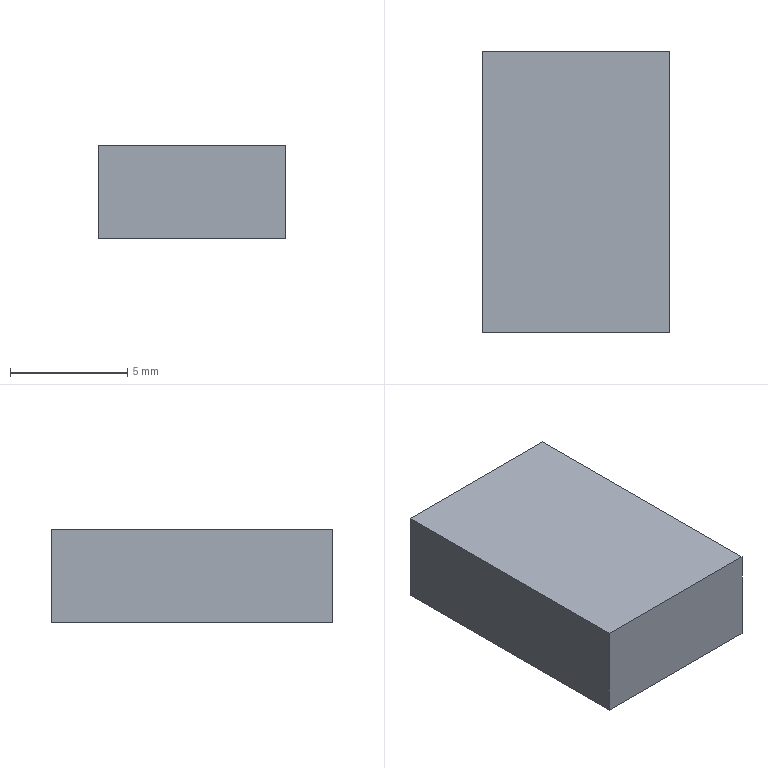Part | SolidWorks | features BaseBody 1 | 1 solid | 6 faces | box 8 x 12 x 4 mm | volume 384 mm3 | plane 6
STEP:
#1=CARTESIAN_POINT('',(4.,-6.,-2.));
#2=VERTEX_POINT('',#1);
#3=CARTESIAN_POINT('',(4.,6.,-2.));
#4=VERTEX_POINT('',#3);
#5=CARTESIAN_POINT('',(4.,-6.,-2.));
#6=DIRECTION('',(0.,1.,0.));
#7=VECTOR('',#6,1000.);
#8=LINE('',#5,#7);
#9=EDGE_CURVE('',#2,#4,#8,.T.);
#10=ORIENTED_EDGE('',*,*,#9,.F.);
#11=CARTESIAN_POINT('',(-4.,-6.,-2.));
#12=VERTEX_POINT('',#11);
#13=CARTESIAN_POINT('',(-4.,-6.,-2.));
#14=DIRECTION('',(1.,0.,0.));
#15=VECTOR('',#14,1000.);
#16=LINE('',#13,#15);
#17=EDGE_CURVE('',#12,#2,#16,.T.);
#18=ORIENTED_EDGE('',*,*,#17,.F.);
#19=CARTESIAN_POINT('',(-4.,6.,-2.));
#20=VERTEX_POINT('',#19);
#21=CARTESIAN_POINT('',(-4.,-6.,-2.));
#22=DIRECTION('',(0.,-1.,0.));
#23=VECTOR('',#22,1000.);
#24=LINE('',#21,#23);
#25=EDGE_CURVE('',#20,#12,#24,.T.);
#26=ORIENTED_EDGE('',*,*,#25,.F.);
#27=CARTESIAN_POINT('',(-4.,6.,-2.));
#28=DIRECTION('',(-1.,0.,0.));
#29=VECTOR('',#28,1000.);
#30=LINE('',#27,#29);
#31=EDGE_CURVE('',#4,#20,#30,.T.);
#32=ORIENTED_EDGE('',*,*,#31,.F.);
#33=EDGE_LOOP('',(#10,#18,#26,#32));
#34=FACE_OUTER_BOUND('',#33,.T.);
#35=CARTESIAN_POINT('',(-4.,-6.,-2.));
#36=DIRECTION('',(0.,0.,1.));
#37=DIRECTION('',(1.,0.,0.));
#38=AXIS2_PLACEMENT_3D('',#35,#36,#37);
#39=PLANE('',#38);
#40=ADVANCED_FACE('',(#34),#39,.F.);
#41=CARTESIAN_POINT('',(-4.,6.,2.));
#42=VERTEX_POINT('',#41);
#43=CARTESIAN_POINT('',(4.,6.,2.));
#44=VERTEX_POINT('',#43);
#45=CARTESIAN_POINT('',(-4.,6.,2.));
#46=DIRECTION('',(1.,0.,0.));
#47=VECTOR('',#46,1000.);
#48=LINE('',#45,#47);
#49=EDGE_CURVE('',#42,#44,#48,.T.);
#50=ORIENTED_EDGE('',*,*,#49,.T.);
#51=CARTESIAN_POINT('',(4.,6.,-2.));
#52=DIRECTION('',(0.,0.,-1.));
#53=VECTOR('',#52,1000.);
#54=LINE('',#51,#53);
#55=EDGE_CURVE('',#44,#4,#54,.T.);
#56=ORIENTED_EDGE('',*,*,#55,.T.);
#57=ORIENTED_EDGE('',*,*,#31,.T.);
#58=CARTESIAN_POINT('',(-4.,6.,-2.));
#59=DIRECTION('',(0.,0.,1.));
#60=VECTOR('',#59,1000.);
#61=LINE('',#58,#60);
#62=EDGE_CURVE('',#20,#42,#61,.T.);
#63=ORIENTED_EDGE('',*,*,#62,.T.);
#64=EDGE_LOOP('',(#50,#56,#57,#63));
#65=FACE_OUTER_BOUND('',#64,.T.);
#66=CARTESIAN_POINT('',(-4.,6.,-2.));
#67=DIRECTION('',(0.,1.,0.));
#68=DIRECTION('',(0.,0.,1.));
#69=AXIS2_PLACEMENT_3D('',#66,#67,#68);
#70=PLANE('',#69);
#71=ADVANCED_FACE('',(#65),#70,.T.);
#72=ORIENTED_EDGE('',*,*,#55,.F.);
#73=CARTESIAN_POINT('',(4.,-6.,2.));
#74=VERTEX_POINT('',#73);
#75=CARTESIAN_POINT('',(4.,-6.,2.));
#76=DIRECTION('',(0.,-1.,0.));
#77=VECTOR('',#76,1000.);
#78=LINE('',#75,#77);
#79=EDGE_CURVE('',#44,#74,#78,.T.);
#80=ORIENTED_EDGE('',*,*,#79,.T.);
#81=CARTESIAN_POINT('',(4.,-6.,-2.));
#82=DIRECTION('',(0.,0.,-1.));
#83=VECTOR('',#82,1000.);
#84=LINE('',#81,#83);
#85=EDGE_CURVE('',#74,#2,#84,.T.);
#86=ORIENTED_EDGE('',*,*,#85,.T.);
#87=ORIENTED_EDGE('',*,*,#9,.T.);
#88=EDGE_LOOP('',(#72,#80,#86,#87));
#89=FACE_OUTER_BOUND('',#88,.T.);
#90=CARTESIAN_POINT('',(4.,-6.,-2.));
#91=DIRECTION('',(1.,0.,0.));
#92=DIRECTION('',(0.,0.,-1.));
#93=AXIS2_PLACEMENT_3D('',#90,#91,#92);
#94=PLANE('',#93);
#95=ADVANCED_FACE('',(#89),#94,.T.);
#96=CARTESIAN_POINT('',(-4.,-6.,2.));
#97=VERTEX_POINT('',#96);
#98=CARTESIAN_POINT('',(-4.,-6.,2.));
#99=DIRECTION('',(1.,0.,0.));
#100=VECTOR('',#99,1000.);
#101=LINE('',#98,#100);
#102=EDGE_CURVE('',#97,#74,#101,.T.);
#103=ORIENTED_EDGE('',*,*,#102,.F.);
#104=CARTESIAN_POINT('',(-4.,-6.,-2.));
#105=DIRECTION('',(0.,0.,1.));
#106=VECTOR('',#105,1000.);
#107=LINE('',#104,#106);
#108=EDGE_CURVE('',#12,#97,#107,.T.);
#109=ORIENTED_EDGE('',*,*,#108,.F.);
#110=ORIENTED_EDGE('',*,*,#17,.T.);
#111=ORIENTED_EDGE('',*,*,#85,.F.);
#112=EDGE_LOOP('',(#103,#109,#110,#111));
#113=FACE_OUTER_BOUND('',#112,.T.);
#114=CARTESIAN_POINT('',(-4.,-6.,-2.));
#115=DIRECTION('',(0.,1.,0.));
#116=DIRECTION('',(0.,0.,1.));
#117=AXIS2_PLACEMENT_3D('',#114,#115,#116);
#118=PLANE('',#117);
#119=ADVANCED_FACE('',(#113),#118,.F.);
#120=ORIENTED_EDGE('',*,*,#62,.F.);
#121=ORIENTED_EDGE('',*,*,#25,.T.);
#122=ORIENTED_EDGE('',*,*,#108,.T.);
#123=CARTESIAN_POINT('',(-4.,-6.,2.));
#124=DIRECTION('',(0.,-1.,0.));
#125=VECTOR('',#124,1000.);
#126=LINE('',#123,#125);
#127=EDGE_CURVE('',#42,#97,#126,.T.);
#128=ORIENTED_EDGE('',*,*,#127,.F.);
#129=EDGE_LOOP('',(#120,#121,#122,#128));
#130=FACE_OUTER_BOUND('',#129,.T.);
#131=CARTESIAN_POINT('',(-4.,-6.,-2.));
#132=DIRECTION('',(1.,0.,0.));
#133=DIRECTION('',(0.,0.,-1.));
#134=AXIS2_PLACEMENT_3D('',#131,#132,#133);
#135=PLANE('',#134);
#136=ADVANCED_FACE('',(#130),#135,.F.);
#137=ORIENTED_EDGE('',*,*,#79,.F.);
#138=ORIENTED_EDGE('',*,*,#49,.F.);
#139=ORIENTED_EDGE('',*,*,#127,.T.);
#140=ORIENTED_EDGE('',*,*,#102,.T.);
#141=EDGE_LOOP('',(#137,#138,#139,#140));
#142=FACE_OUTER_BOUND('',#141,.T.);
#143=CARTESIAN_POINT('',(-4.,-6.,2.));
#144=DIRECTION('',(0.,0.,1.));
#145=DIRECTION('',(1.,0.,0.));
#146=AXIS2_PLACEMENT_3D('',#143,#144,#145);
#147=PLANE('',#146);
#148=ADVANCED_FACE('',(#142),#147,.T.);
#149=CLOSED_SHELL('',(#40,#71,#95,#119,#136,#148));
#150=MANIFOLD_SOLID_BREP('',#149);
#151=CARTESIAN_POINT('',(0.,0.,0.));
#152=DIRECTION('',(0.,0.,1.));
#153=DIRECTION('',(1.,0.,0.));
#154=AXIS2_PLACEMENT_3D('',#151,#152,#153);
#155=(LENGTH_UNIT()NAMED_UNIT(*)SI_UNIT(.MILLI.,.METRE.));
#156=UNCERTAINTY_MEASURE_WITH_UNIT(LENGTH_MEASURE(0.00001),#155,'','');
#157=(NAMED_UNIT(*)PLANE_ANGLE_UNIT()SI_UNIT($,.RADIAN.));
#158=(NAMED_UNIT(*)SI_UNIT($,.STERADIAN.)SOLID_ANGLE_UNIT());
#159=(GEOMETRIC_REPRESENTATION_CONTEXT(3)GLOBAL_UNCERTAINTY_ASSIGNED_CONTEXT((#156))GLOBAL_UNIT_ASSIGNED_CONTEXT((#155,#157,#158))REPRESENTATION_CONTEXT('',''));
#160=ADVANCED_BREP_SHAPE_REPRESENTATION('',(#150,#154),#159);